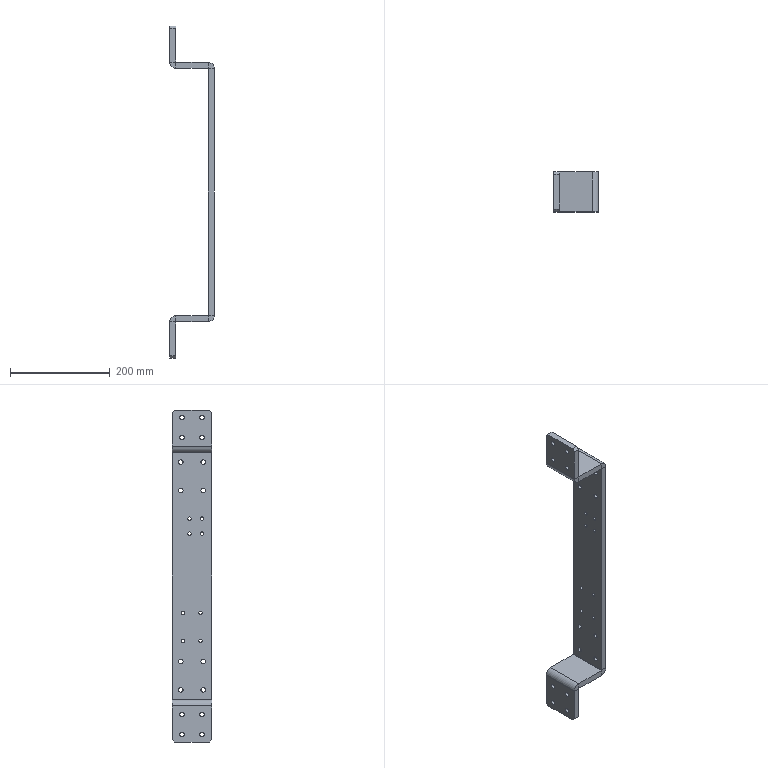Part | SolidWorks | features HoleWzd 4, EdgeFlange 2, Chamfer 1, FlatPattern 1, MirrorPattern 1, SMBaseFlange 1, SheetMetal 1 | 1 solid | 90 faces | box 90 x 80 x 666 mm | volume 761508 mm3 | cylinder 56 | plane 34 | commonest cylinder face diameters 9 x32 7 x16 1.473 x4 25.473 x4